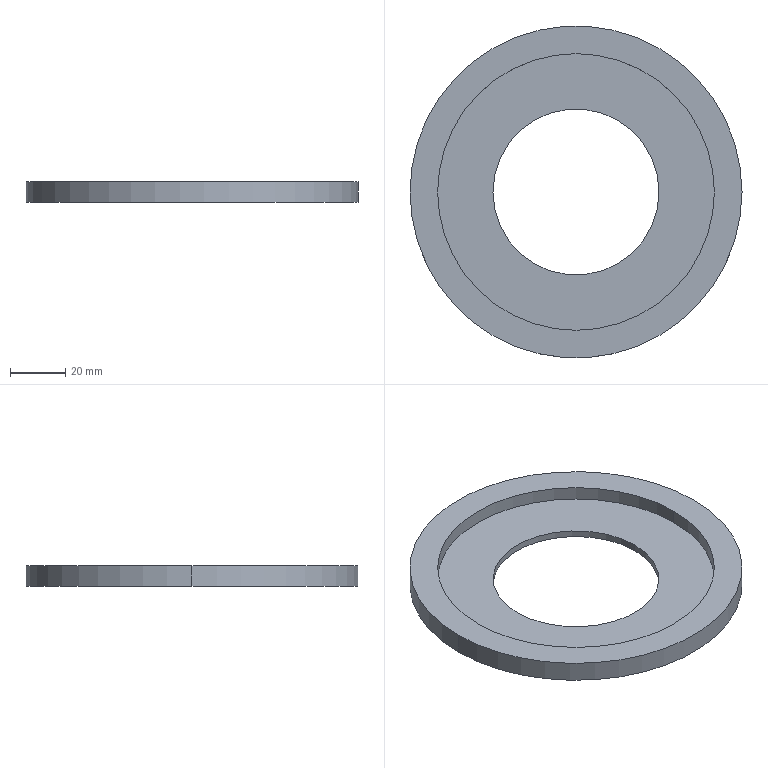Part | SolidWorks | features RefAxis 4, ICE 2, Extrusion 1 | 1 solid | 9 faces | box 120 x 120 x 7.5 mm | volume 38485 mm3 | cylinder 6 | plane 3 | commonest cylinder face diameters 60 x2 100 x2 120 x2
STEP:
#1=CARTESIAN_POINT('',(30.,0.,2.5));
#2=VERTEX_POINT('',#1);
#3=CARTESIAN_POINT('',(-30.,0.,2.5));
#4=VERTEX_POINT('',#3);
#5=CARTESIAN_POINT('',(0.,0.,2.5));
#6=DIRECTION('',(0.,0.,-1.));
#7=DIRECTION('',(-1.,0.,0.));
#8=AXIS2_PLACEMENT_3D('',#5,#6,#7);
#9=CIRCLE('',#8,30.);
#10=EDGE_CURVE('',#2,#4,#9,.T.);
#11=ORIENTED_EDGE('',*,*,#10,.F.);
#12=CARTESIAN_POINT('',(30.,0.,0.));
#13=VERTEX_POINT('',#12);
#14=CARTESIAN_POINT('',(30.,0.,10.));
#15=DIRECTION('',(0.,0.,-1.));
#16=VECTOR('',#15,1000.);
#17=LINE('',#14,#16);
#18=EDGE_CURVE('',#2,#13,#17,.T.);
#19=ORIENTED_EDGE('',*,*,#18,.T.);
#20=CARTESIAN_POINT('',(-30.,0.,0.));
#21=VERTEX_POINT('',#20);
#22=CARTESIAN_POINT('',(0.,0.,0.));
#23=DIRECTION('',(0.,0.,-1.));
#24=DIRECTION('',(-1.,0.,0.));
#25=AXIS2_PLACEMENT_3D('',#22,#23,#24);
#26=CIRCLE('',#25,30.);
#27=EDGE_CURVE('',#13,#21,#26,.T.);
#28=ORIENTED_EDGE('',*,*,#27,.T.);
#29=CARTESIAN_POINT('',(-30.,0.,10.));
#30=DIRECTION('',(0.,0.,-1.));
#31=VECTOR('',#30,1000.);
#32=LINE('',#29,#31);
#33=EDGE_CURVE('',#4,#21,#32,.T.);
#34=ORIENTED_EDGE('',*,*,#33,.F.);
#35=EDGE_LOOP('',(#11,#19,#28,#34));
#36=FACE_OUTER_BOUND('',#35,.T.);
#37=CARTESIAN_POINT('',(0.,0.,10.));
#38=DIRECTION('',(0.,0.,-1.));
#39=DIRECTION('',(-1.,0.,0.));
#40=AXIS2_PLACEMENT_3D('',#37,#38,#39);
#41=CYLINDRICAL_SURFACE('',#40,30.);
#42=ADVANCED_FACE('',(#36),#41,.F.);
#43=CARTESIAN_POINT('',(60.,0.,7.5));
#44=VERTEX_POINT('',#43);
#45=CARTESIAN_POINT('',(-60.,0.,7.5));
#46=VERTEX_POINT('',#45);
#47=CARTESIAN_POINT('',(0.,0.,7.5));
#48=DIRECTION('',(0.,0.,1.));
#49=DIRECTION('',(1.,0.,0.));
#50=AXIS2_PLACEMENT_3D('',#47,#48,#49);
#51=CIRCLE('',#50,60.);
#52=EDGE_CURVE('',#44,#46,#51,.T.);
#53=ORIENTED_EDGE('',*,*,#52,.F.);
#54=CARTESIAN_POINT('',(60.,0.,0.));
#55=VERTEX_POINT('',#54);
#56=CARTESIAN_POINT('',(60.,0.,7.5));
#57=DIRECTION('',(0.,0.,-1.));
#58=VECTOR('',#57,1000.);
#59=LINE('',#56,#58);
#60=EDGE_CURVE('',#44,#55,#59,.T.);
#61=ORIENTED_EDGE('',*,*,#60,.T.);
#62=CARTESIAN_POINT('',(-60.,0.,0.));
#63=VERTEX_POINT('',#62);
#64=CARTESIAN_POINT('',(0.,0.,0.));
#65=DIRECTION('',(0.,0.,1.));
#66=DIRECTION('',(1.,0.,0.));
#67=AXIS2_PLACEMENT_3D('',#64,#65,#66);
#68=CIRCLE('',#67,60.);
#69=EDGE_CURVE('',#55,#63,#68,.T.);
#70=ORIENTED_EDGE('',*,*,#69,.T.);
#71=CARTESIAN_POINT('',(-60.,0.,7.5));
#72=DIRECTION('',(0.,0.,-1.));
#73=VECTOR('',#72,1000.);
#74=LINE('',#71,#73);
#75=EDGE_CURVE('',#46,#63,#74,.T.);
#76=ORIENTED_EDGE('',*,*,#75,.F.);
#77=EDGE_LOOP('',(#53,#61,#70,#76));
#78=FACE_OUTER_BOUND('',#77,.T.);
#79=CARTESIAN_POINT('',(0.,0.,7.5));
#80=DIRECTION('',(0.,0.,-1.));
#81=DIRECTION('',(-1.,0.,0.));
#82=AXIS2_PLACEMENT_3D('',#79,#80,#81);
#83=CYLINDRICAL_SURFACE('',#82,60.);
#84=ADVANCED_FACE('',(#78),#83,.T.);
#85=CARTESIAN_POINT('',(-50.,0.,7.5));
#86=VERTEX_POINT('',#85);
#87=CARTESIAN_POINT('',(50.,0.,7.5));
#88=VERTEX_POINT('',#87);
#89=CARTESIAN_POINT('',(0.,0.,7.5));
#90=DIRECTION('',(0.,0.,1.));
#91=DIRECTION('',(1.,0.,0.));
#92=AXIS2_PLACEMENT_3D('',#89,#90,#91);
#93=CIRCLE('',#92,50.);
#94=EDGE_CURVE('',#86,#88,#93,.T.);
#95=ORIENTED_EDGE('',*,*,#94,.T.);
#96=CARTESIAN_POINT('',(50.,0.,2.5));
#97=VERTEX_POINT('',#96);
#98=CARTESIAN_POINT('',(50.,0.,7.5));
#99=DIRECTION('',(0.,0.,-1.));
#100=VECTOR('',#99,1000.);
#101=LINE('',#98,#100);
#102=EDGE_CURVE('',#88,#97,#101,.T.);
#103=ORIENTED_EDGE('',*,*,#102,.T.);
#104=CARTESIAN_POINT('',(-50.,0.,2.5));
#105=VERTEX_POINT('',#104);
#106=CARTESIAN_POINT('',(0.,0.,2.5));
#107=DIRECTION('',(0.,0.,-1.));
#108=DIRECTION('',(-1.,0.,0.));
#109=AXIS2_PLACEMENT_3D('',#106,#107,#108);
#110=CIRCLE('',#109,50.);
#111=EDGE_CURVE('',#97,#105,#110,.T.);
#112=ORIENTED_EDGE('',*,*,#111,.T.);
#113=CARTESIAN_POINT('',(-50.,0.,7.5));
#114=DIRECTION('',(0.,0.,-1.));
#115=VECTOR('',#114,1000.);
#116=LINE('',#113,#115);
#117=EDGE_CURVE('',#86,#105,#116,.T.);
#118=ORIENTED_EDGE('',*,*,#117,.F.);
#119=EDGE_LOOP('',(#95,#103,#112,#118));
#120=FACE_OUTER_BOUND('',#119,.T.);
#121=CARTESIAN_POINT('',(0.,0.,7.5));
#122=DIRECTION('',(0.,0.,-1.));
#123=DIRECTION('',(-1.,0.,0.));
#124=AXIS2_PLACEMENT_3D('',#121,#122,#123);
#125=CYLINDRICAL_SURFACE('',#124,50.);
#126=ADVANCED_FACE('',(#120),#125,.F.);
#127=ORIENTED_EDGE('',*,*,#102,.F.);
#128=CARTESIAN_POINT('',(0.,0.,7.5));
#129=DIRECTION('',(0.,0.,1.));
#130=DIRECTION('',(1.,0.,0.));
#131=AXIS2_PLACEMENT_3D('',#128,#129,#130);
#132=CIRCLE('',#131,50.);
#133=EDGE_CURVE('',#88,#86,#132,.T.);
#134=ORIENTED_EDGE('',*,*,#133,.T.);
#135=ORIENTED_EDGE('',*,*,#117,.T.);
#136=CARTESIAN_POINT('',(0.,0.,2.5));
#137=DIRECTION('',(0.,0.,-1.));
#138=DIRECTION('',(-1.,0.,0.));
#139=AXIS2_PLACEMENT_3D('',#136,#137,#138);
#140=CIRCLE('',#139,50.);
#141=EDGE_CURVE('',#105,#97,#140,.T.);
#142=ORIENTED_EDGE('',*,*,#141,.T.);
#143=EDGE_LOOP('',(#127,#134,#135,#142));
#144=FACE_OUTER_BOUND('',#143,.T.);
#145=CARTESIAN_POINT('',(0.,0.,7.5));
#146=DIRECTION('',(0.,0.,-1.));
#147=DIRECTION('',(-1.,0.,0.));
#148=AXIS2_PLACEMENT_3D('',#145,#146,#147);
#149=CYLINDRICAL_SURFACE('',#148,50.);
#150=ADVANCED_FACE('',(#144),#149,.F.);
#151=CARTESIAN_POINT('',(0.,0.,7.5));
#152=DIRECTION('',(0.,0.,1.));
#153=DIRECTION('',(1.,0.,0.));
#154=AXIS2_PLACEMENT_3D('',#151,#152,#153);
#155=CIRCLE('',#154,60.);
#156=EDGE_CURVE('',#46,#44,#155,.T.);
#157=ORIENTED_EDGE('',*,*,#156,.T.);
#158=ORIENTED_EDGE('',*,*,#52,.T.);
#159=EDGE_LOOP('',(#157,#158));
#160=FACE_OUTER_BOUND('',#159,.T.);
#161=ORIENTED_EDGE('',*,*,#94,.F.);
#162=ORIENTED_EDGE('',*,*,#133,.F.);
#163=EDGE_LOOP('',(#161,#162));
#164=FACE_BOUND('',#163,.T.);
#165=CARTESIAN_POINT('',(0.,0.,7.5));
#166=DIRECTION('',(0.,0.,1.));
#167=DIRECTION('',(1.,0.,0.));
#168=AXIS2_PLACEMENT_3D('',#165,#166,#167);
#169=PLANE('',#168);
#170=ADVANCED_FACE('',(#160,#164),#169,.T.);
#171=CARTESIAN_POINT('',(0.,0.,0.));
#172=DIRECTION('',(0.,0.,-1.));
#173=DIRECTION('',(-1.,0.,0.));
#174=AXIS2_PLACEMENT_3D('',#171,#172,#173);
#175=CIRCLE('',#174,30.);
#176=EDGE_CURVE('',#21,#13,#175,.T.);
#177=ORIENTED_EDGE('',*,*,#176,.F.);
#178=ORIENTED_EDGE('',*,*,#27,.F.);
#179=EDGE_LOOP('',(#177,#178));
#180=FACE_BOUND('',#179,.T.);
#181=CARTESIAN_POINT('',(0.,0.,0.));
#182=DIRECTION('',(0.,0.,1.));
#183=DIRECTION('',(1.,0.,0.));
#184=AXIS2_PLACEMENT_3D('',#181,#182,#183);
#185=CIRCLE('',#184,60.);
#186=EDGE_CURVE('',#63,#55,#185,.T.);
#187=ORIENTED_EDGE('',*,*,#186,.F.);
#188=ORIENTED_EDGE('',*,*,#69,.F.);
#189=EDGE_LOOP('',(#187,#188));
#190=FACE_OUTER_BOUND('',#189,.T.);
#191=CARTESIAN_POINT('',(0.,0.,0.));
#192=DIRECTION('',(0.,0.,1.));
#193=DIRECTION('',(1.,0.,0.));
#194=AXIS2_PLACEMENT_3D('',#191,#192,#193);
#195=PLANE('',#194);
#196=ADVANCED_FACE('',(#180,#190),#195,.F.);
#197=ORIENTED_EDGE('',*,*,#60,.F.);
#198=ORIENTED_EDGE('',*,*,#156,.F.);
#199=ORIENTED_EDGE('',*,*,#75,.T.);
#200=ORIENTED_EDGE('',*,*,#186,.T.);
#201=EDGE_LOOP('',(#197,#198,#199,#200));
#202=FACE_OUTER_BOUND('',#201,.T.);
#203=CARTESIAN_POINT('',(0.,0.,7.5));
#204=DIRECTION('',(0.,0.,-1.));
#205=DIRECTION('',(-1.,0.,0.));
#206=AXIS2_PLACEMENT_3D('',#203,#204,#205);
#207=CYLINDRICAL_SURFACE('',#206,60.);
#208=ADVANCED_FACE('',(#202),#207,.T.);
#209=CARTESIAN_POINT('',(0.,0.,2.5));
#210=DIRECTION('',(0.,0.,-1.));
#211=DIRECTION('',(-1.,0.,0.));
#212=AXIS2_PLACEMENT_3D('',#209,#210,#211);
#213=CIRCLE('',#212,30.);
#214=EDGE_CURVE('',#4,#2,#213,.T.);
#215=ORIENTED_EDGE('',*,*,#214,.T.);
#216=ORIENTED_EDGE('',*,*,#10,.T.);
#217=EDGE_LOOP('',(#215,#216));
#218=FACE_BOUND('',#217,.T.);
#219=ORIENTED_EDGE('',*,*,#141,.F.);
#220=ORIENTED_EDGE('',*,*,#111,.F.);
#221=EDGE_LOOP('',(#219,#220));
#222=FACE_OUTER_BOUND('',#221,.T.);
#223=CARTESIAN_POINT('',(0.,0.,2.5));
#224=DIRECTION('',(0.,0.,-1.));
#225=DIRECTION('',(-1.,0.,0.));
#226=AXIS2_PLACEMENT_3D('',#223,#224,#225);
#227=PLANE('',#226);
#228=ADVANCED_FACE('',(#218,#222),#227,.F.);
#229=ORIENTED_EDGE('',*,*,#18,.F.);
#230=ORIENTED_EDGE('',*,*,#214,.F.);
#231=ORIENTED_EDGE('',*,*,#33,.T.);
#232=ORIENTED_EDGE('',*,*,#176,.T.);
#233=EDGE_LOOP('',(#229,#230,#231,#232));
#234=FACE_OUTER_BOUND('',#233,.T.);
#235=CARTESIAN_POINT('',(0.,0.,10.));
#236=DIRECTION('',(0.,0.,-1.));
#237=DIRECTION('',(-1.,0.,0.));
#238=AXIS2_PLACEMENT_3D('',#235,#236,#237);
#239=CYLINDRICAL_SURFACE('',#238,30.);
#240=ADVANCED_FACE('',(#234),#239,.F.);
#241=CLOSED_SHELL('',(#42,#84,#126,#150,#170,#196,#208,#228,#240));
#242=MANIFOLD_SOLID_BREP('',#241);
#243=CARTESIAN_POINT('',(0.,0.,0.));
#244=DIRECTION('',(0.,0.,1.));
#245=DIRECTION('',(1.,0.,0.));
#246=AXIS2_PLACEMENT_3D('',#243,#244,#245);
#247=(LENGTH_UNIT()NAMED_UNIT(*)SI_UNIT(.MILLI.,.METRE.));
#248=UNCERTAINTY_MEASURE_WITH_UNIT(LENGTH_MEASURE(0.00001),#247,'','');
#249=(NAMED_UNIT(*)PLANE_ANGLE_UNIT()SI_UNIT($,.RADIAN.));
#250=(NAMED_UNIT(*)SI_UNIT($,.STERADIAN.)SOLID_ANGLE_UNIT());
#251=(GEOMETRIC_REPRESENTATION_CONTEXT(3)GLOBAL_UNCERTAINTY_ASSIGNED_CONTEXT((#248))GLOBAL_UNIT_ASSIGNED_CONTEXT((#247,#249,#250))REPRESENTATION_CONTEXT('',''));
#252=ADVANCED_BREP_SHAPE_REPRESENTATION('',(#242,#246),#251);